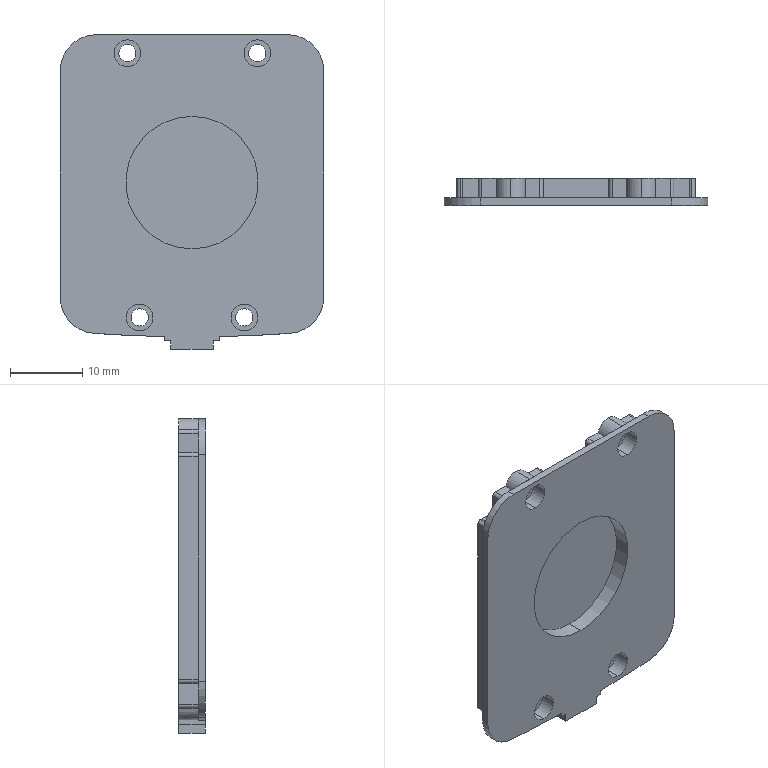Part | SolidWorks | features ICE 7, Extrusion 1, RevCut 1 | 1 solid | 135 faces | box 36.5 x 3.7 x 43.598 mm | volume 2859 mm3 | plane 79 | cylinder 56 | commonest cylinder face diameters 1 x12 2.4 x8 3.7 x8 2 x4 3 x4 4.2 x4